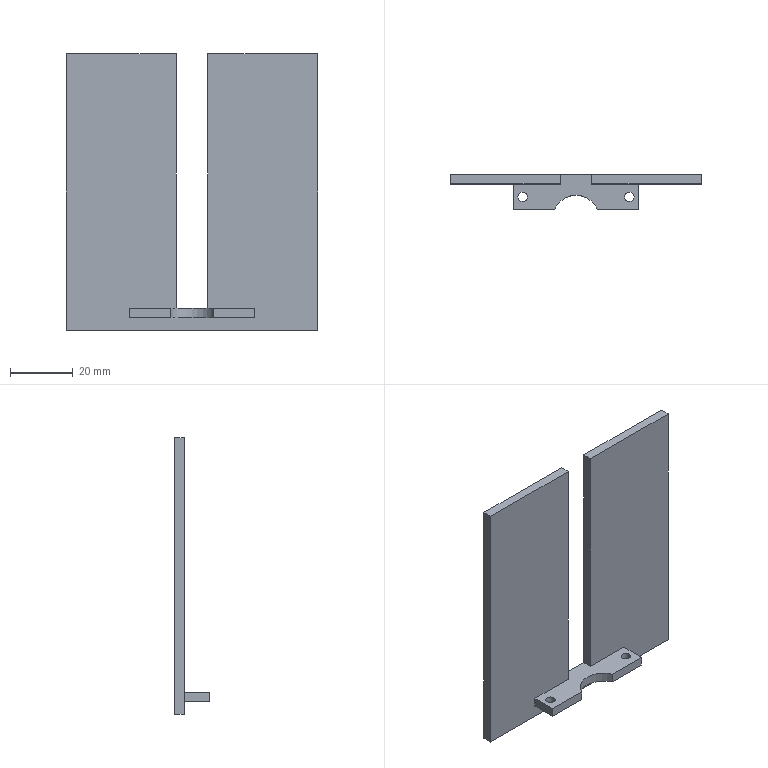Part | SolidWorks | features Extrusion 1, ICE 1 | 1 solid | 20 faces | box 80 x 11 x 88 mm | volume 19474 mm3 | plane 15 | cylinder 5 | commonest cylinder face diameters 3 x4 15 x1
STEP:
#1=CARTESIAN_POINT('',(15.5,7.,3.));
#2=VERTEX_POINT('',#1);
#3=CARTESIAN_POINT('',(18.5,7.,3.));
#4=VERTEX_POINT('',#3);
#5=CARTESIAN_POINT('',(17.,7.,3.));
#6=DIRECTION('',(0.,0.,1.));
#7=DIRECTION('',(1.,0.,0.));
#8=AXIS2_PLACEMENT_3D('',#5,#6,#7);
#9=CIRCLE('',#8,1.5);
#10=EDGE_CURVE('',#2,#4,#9,.T.);
#11=ORIENTED_EDGE('',*,*,#10,.T.);
#12=CARTESIAN_POINT('',(18.5,7.,0.));
#13=VERTEX_POINT('',#12);
#14=CARTESIAN_POINT('',(18.5,7.,3.));
#15=DIRECTION('',(0.,0.,-1.));
#16=VECTOR('',#15,1000.);
#17=LINE('',#14,#16);
#18=EDGE_CURVE('',#4,#13,#17,.T.);
#19=ORIENTED_EDGE('',*,*,#18,.T.);
#20=CARTESIAN_POINT('',(15.5,7.,0.));
#21=VERTEX_POINT('',#20);
#22=CARTESIAN_POINT('',(17.,7.,0.));
#23=DIRECTION('',(0.,0.,1.));
#24=DIRECTION('',(1.,0.,0.));
#25=AXIS2_PLACEMENT_3D('',#22,#23,#24);
#26=CIRCLE('',#25,1.5);
#27=EDGE_CURVE('',#21,#13,#26,.T.);
#28=ORIENTED_EDGE('',*,*,#27,.F.);
#29=CARTESIAN_POINT('',(15.5,7.,3.));
#30=DIRECTION('',(0.,0.,-1.));
#31=VECTOR('',#30,1000.);
#32=LINE('',#29,#31);
#33=EDGE_CURVE('',#2,#21,#32,.T.);
#34=ORIENTED_EDGE('',*,*,#33,.F.);
#35=EDGE_LOOP('',(#11,#19,#28,#34));
#36=FACE_OUTER_BOUND('',#35,.T.);
#37=CARTESIAN_POINT('',(17.,7.,3.));
#38=DIRECTION('',(0.,0.,-1.));
#39=DIRECTION('',(-1.,0.,0.));
#40=AXIS2_PLACEMENT_3D('',#37,#38,#39);
#41=CYLINDRICAL_SURFACE('',#40,1.5);
#42=ADVANCED_FACE('',(#36),#41,.F.);
#43=CARTESIAN_POINT('',(-18.5,7.,3.));
#44=VERTEX_POINT('',#43);
#45=CARTESIAN_POINT('',(-15.5,7.,3.));
#46=VERTEX_POINT('',#45);
#47=CARTESIAN_POINT('',(-17.,7.,3.));
#48=DIRECTION('',(0.,0.,1.));
#49=DIRECTION('',(1.,0.,0.));
#50=AXIS2_PLACEMENT_3D('',#47,#48,#49);
#51=CIRCLE('',#50,1.5);
#52=EDGE_CURVE('',#44,#46,#51,.T.);
#53=ORIENTED_EDGE('',*,*,#52,.T.);
#54=CARTESIAN_POINT('',(-15.5,7.,0.));
#55=VERTEX_POINT('',#54);
#56=CARTESIAN_POINT('',(-15.5,7.,3.));
#57=DIRECTION('',(0.,0.,-1.));
#58=VECTOR('',#57,1000.);
#59=LINE('',#56,#58);
#60=EDGE_CURVE('',#46,#55,#59,.T.);
#61=ORIENTED_EDGE('',*,*,#60,.T.);
#62=CARTESIAN_POINT('',(-18.5,7.,0.));
#63=VERTEX_POINT('',#62);
#64=CARTESIAN_POINT('',(-17.,7.,0.));
#65=DIRECTION('',(0.,0.,1.));
#66=DIRECTION('',(1.,0.,0.));
#67=AXIS2_PLACEMENT_3D('',#64,#65,#66);
#68=CIRCLE('',#67,1.5);
#69=EDGE_CURVE('',#63,#55,#68,.T.);
#70=ORIENTED_EDGE('',*,*,#69,.F.);
#71=CARTESIAN_POINT('',(-18.5,7.,3.));
#72=DIRECTION('',(0.,0.,-1.));
#73=VECTOR('',#72,1000.);
#74=LINE('',#71,#73);
#75=EDGE_CURVE('',#44,#63,#74,.T.);
#76=ORIENTED_EDGE('',*,*,#75,.F.);
#77=EDGE_LOOP('',(#53,#61,#70,#76));
#78=FACE_OUTER_BOUND('',#77,.T.);
#79=CARTESIAN_POINT('',(-17.,7.,3.));
#80=DIRECTION('',(0.,0.,-1.));
#81=DIRECTION('',(-1.,0.,0.));
#82=AXIS2_PLACEMENT_3D('',#79,#80,#81);
#83=CYLINDRICAL_SURFACE('',#82,1.5);
#84=ADVANCED_FACE('',(#78),#83,.F.);
#85=ORIENTED_EDGE('',*,*,#52,.F.);
#86=CARTESIAN_POINT('',(-17.,7.,3.));
#87=DIRECTION('',(0.,0.,1.));
#88=DIRECTION('',(1.,0.,0.));
#89=AXIS2_PLACEMENT_3D('',#86,#87,#88);
#90=CIRCLE('',#89,1.5);
#91=EDGE_CURVE('',#46,#44,#90,.T.);
#92=ORIENTED_EDGE('',*,*,#91,.F.);
#93=EDGE_LOOP('',(#85,#92));
#94=FACE_BOUND('',#93,.T.);
#95=CARTESIAN_POINT('',(20.,3.,3.));
#96=VERTEX_POINT('',#95);
#97=CARTESIAN_POINT('',(20.,11.,3.));
#98=VERTEX_POINT('',#97);
#99=CARTESIAN_POINT('',(20.,3.,3.));
#100=DIRECTION('',(0.,1.,0.));
#101=VECTOR('',#100,1000.);
#102=LINE('',#99,#101);
#103=EDGE_CURVE('',#96,#98,#102,.T.);
#104=ORIENTED_EDGE('',*,*,#103,.T.);
#105=CARTESIAN_POINT('',(5.,11.,3.));
#106=VERTEX_POINT('',#105);
#107=CARTESIAN_POINT('',(-20.,11.,3.));
#108=DIRECTION('',(-1.,0.,0.));
#109=VECTOR('',#108,1000.);
#110=LINE('',#107,#109);
#111=EDGE_CURVE('',#98,#106,#110,.T.);
#112=ORIENTED_EDGE('',*,*,#111,.T.);
#113=CARTESIAN_POINT('',(5.,14.,3.));
#114=VERTEX_POINT('',#113);
#115=CARTESIAN_POINT('',(5.,14.,3.));
#116=DIRECTION('',(0.,-1.,0.));
#117=VECTOR('',#116,1000.);
#118=LINE('',#115,#117);
#119=EDGE_CURVE('',#114,#106,#118,.T.);
#120=ORIENTED_EDGE('',*,*,#119,.F.);
#121=CARTESIAN_POINT('',(-5.,14.,3.));
#122=VERTEX_POINT('',#121);
#123=CARTESIAN_POINT('',(-5.,14.,3.));
#124=DIRECTION('',(1.,0.,0.));
#125=VECTOR('',#124,1000.);
#126=LINE('',#123,#125);
#127=EDGE_CURVE('',#122,#114,#126,.T.);
#128=ORIENTED_EDGE('',*,*,#127,.F.);
#129=CARTESIAN_POINT('',(-5.,11.,3.));
#130=VERTEX_POINT('',#129);
#131=CARTESIAN_POINT('',(-5.,14.,3.));
#132=DIRECTION('',(0.,-1.,0.));
#133=VECTOR('',#132,1000.);
#134=LINE('',#131,#133);
#135=EDGE_CURVE('',#122,#130,#134,.T.);
#136=ORIENTED_EDGE('',*,*,#135,.T.);
#137=CARTESIAN_POINT('',(-20.,11.,3.));
#138=VERTEX_POINT('',#137);
#139=CARTESIAN_POINT('',(-20.,11.,3.));
#140=DIRECTION('',(-1.,0.,0.));
#141=VECTOR('',#140,1000.);
#142=LINE('',#139,#141);
#143=EDGE_CURVE('',#130,#138,#142,.T.);
#144=ORIENTED_EDGE('',*,*,#143,.T.);
#145=CARTESIAN_POINT('',(-20.,3.,3.));
#146=VERTEX_POINT('',#145);
#147=CARTESIAN_POINT('',(-20.,3.,3.));
#148=DIRECTION('',(0.,-1.,0.));
#149=VECTOR('',#148,1000.);
#150=LINE('',#147,#149);
#151=EDGE_CURVE('',#138,#146,#150,.T.);
#152=ORIENTED_EDGE('',*,*,#151,.T.);
#153=CARTESIAN_POINT('',(-6.874,3.,3.));
#154=VERTEX_POINT('',#153);
#155=CARTESIAN_POINT('',(-20.,3.,3.));
#156=DIRECTION('',(1.,0.,0.));
#157=VECTOR('',#156,1000.);
#158=LINE('',#155,#157);
#159=EDGE_CURVE('',#146,#154,#158,.T.);
#160=ORIENTED_EDGE('',*,*,#159,.T.);
#161=CARTESIAN_POINT('',(6.874,3.,3.));
#162=VERTEX_POINT('',#161);
#163=CARTESIAN_POINT('',(0.,0.,3.));
#164=DIRECTION('',(0.,0.,-1.));
#165=DIRECTION('',(1.,0.,0.));
#166=AXIS2_PLACEMENT_3D('',#163,#164,#165);
#167=CIRCLE('',#166,7.5);
#168=EDGE_CURVE('',#154,#162,#167,.T.);
#169=ORIENTED_EDGE('',*,*,#168,.T.);
#170=CARTESIAN_POINT('',(6.874,3.,3.));
#171=DIRECTION('',(1.,0.,0.));
#172=VECTOR('',#171,1000.);
#173=LINE('',#170,#172);
#174=EDGE_CURVE('',#162,#96,#173,.T.);
#175=ORIENTED_EDGE('',*,*,#174,.T.);
#176=EDGE_LOOP('',(#104,#112,#120,#128,#136,#144,#152,#160,#169,#175));
#177=FACE_OUTER_BOUND('',#176,.T.);
#178=ORIENTED_EDGE('',*,*,#10,.F.);
#179=CARTESIAN_POINT('',(17.,7.,3.));
#180=DIRECTION('',(0.,0.,1.));
#181=DIRECTION('',(1.,0.,0.));
#182=AXIS2_PLACEMENT_3D('',#179,#180,#181);
#183=CIRCLE('',#182,1.5);
#184=EDGE_CURVE('',#4,#2,#183,.T.);
#185=ORIENTED_EDGE('',*,*,#184,.F.);
#186=EDGE_LOOP('',(#178,#185));
#187=FACE_BOUND('',#186,.T.);
#188=CARTESIAN_POINT('',(0.,0.,3.));
#189=DIRECTION('',(0.,0.,1.));
#190=DIRECTION('',(1.,0.,0.));
#191=AXIS2_PLACEMENT_3D('',#188,#189,#190);
#192=PLANE('',#191);
#193=ADVANCED_FACE('',(#94,#177,#187),#192,.T.);
#194=CARTESIAN_POINT('',(20.,3.,0.));
#195=VERTEX_POINT('',#194);
#196=CARTESIAN_POINT('',(20.,11.,0.));
#197=VERTEX_POINT('',#196);
#198=CARTESIAN_POINT('',(20.,3.,0.));
#199=DIRECTION('',(0.,1.,0.));
#200=VECTOR('',#199,1000.);
#201=LINE('',#198,#200);
#202=EDGE_CURVE('',#195,#197,#201,.T.);
#203=ORIENTED_EDGE('',*,*,#202,.F.);
#204=CARTESIAN_POINT('',(6.874,3.,0.));
#205=VERTEX_POINT('',#204);
#206=CARTESIAN_POINT('',(6.874,3.,0.));
#207=DIRECTION('',(1.,0.,0.));
#208=VECTOR('',#207,1000.);
#209=LINE('',#206,#208);
#210=EDGE_CURVE('',#205,#195,#209,.T.);
#211=ORIENTED_EDGE('',*,*,#210,.F.);
#212=CARTESIAN_POINT('',(-6.874,3.,0.));
#213=VERTEX_POINT('',#212);
#214=CARTESIAN_POINT('',(0.,0.,0.));
#215=DIRECTION('',(0.,0.,-1.));
#216=DIRECTION('',(1.,0.,0.));
#217=AXIS2_PLACEMENT_3D('',#214,#215,#216);
#218=CIRCLE('',#217,7.5);
#219=EDGE_CURVE('',#213,#205,#218,.T.);
#220=ORIENTED_EDGE('',*,*,#219,.F.);
#221=CARTESIAN_POINT('',(-20.,3.,0.));
#222=VERTEX_POINT('',#221);
#223=CARTESIAN_POINT('',(-20.,3.,0.));
#224=DIRECTION('',(1.,0.,0.));
#225=VECTOR('',#224,1000.);
#226=LINE('',#223,#225);
#227=EDGE_CURVE('',#222,#213,#226,.T.);
#228=ORIENTED_EDGE('',*,*,#227,.F.);
#229=CARTESIAN_POINT('',(-20.,11.,0.));
#230=VERTEX_POINT('',#229);
#231=CARTESIAN_POINT('',(-20.,3.,0.));
#232=DIRECTION('',(0.,-1.,0.));
#233=VECTOR('',#232,1000.);
#234=LINE('',#231,#233);
#235=EDGE_CURVE('',#230,#222,#234,.T.);
#236=ORIENTED_EDGE('',*,*,#235,.F.);
#237=CARTESIAN_POINT('',(-20.,11.,0.));
#238=DIRECTION('',(-1.,0.,0.));
#239=VECTOR('',#238,1000.);
#240=LINE('',#237,#239);
#241=EDGE_CURVE('',#197,#230,#240,.T.);
#242=ORIENTED_EDGE('',*,*,#241,.F.);
#243=EDGE_LOOP('',(#203,#211,#220,#228,#236,#242));
#244=FACE_OUTER_BOUND('',#243,.T.);
#245=ORIENTED_EDGE('',*,*,#69,.T.);
#246=CARTESIAN_POINT('',(-17.,7.,0.));
#247=DIRECTION('',(0.,0.,1.));
#248=DIRECTION('',(1.,0.,0.));
#249=AXIS2_PLACEMENT_3D('',#246,#247,#248);
#250=CIRCLE('',#249,1.5);
#251=EDGE_CURVE('',#55,#63,#250,.T.);
#252=ORIENTED_EDGE('',*,*,#251,.T.);
#253=EDGE_LOOP('',(#245,#252));
#254=FACE_BOUND('',#253,.T.);
#255=ORIENTED_EDGE('',*,*,#27,.T.);
#256=CARTESIAN_POINT('',(17.,7.,0.));
#257=DIRECTION('',(0.,0.,1.));
#258=DIRECTION('',(1.,0.,0.));
#259=AXIS2_PLACEMENT_3D('',#256,#257,#258);
#260=CIRCLE('',#259,1.5);
#261=EDGE_CURVE('',#13,#21,#260,.T.);
#262=ORIENTED_EDGE('',*,*,#261,.T.);
#263=EDGE_LOOP('',(#255,#262));
#264=FACE_BOUND('',#263,.T.);
#265=CARTESIAN_POINT('',(0.,0.,0.));
#266=DIRECTION('',(0.,0.,1.));
#267=DIRECTION('',(1.,0.,0.));
#268=AXIS2_PLACEMENT_3D('',#265,#266,#267);
#269=PLANE('',#268);
#270=ADVANCED_FACE('',(#244,#254,#264),#269,.F.);
#271=ORIENTED_EDGE('',*,*,#202,.T.);
#272=CARTESIAN_POINT('',(20.,11.,3.));
#273=DIRECTION('',(0.,0.,-1.));
#274=VECTOR('',#273,1000.);
#275=LINE('',#272,#274);
#276=EDGE_CURVE('',#98,#197,#275,.T.);
#277=ORIENTED_EDGE('',*,*,#276,.F.);
#278=ORIENTED_EDGE('',*,*,#103,.F.);
#279=CARTESIAN_POINT('',(20.,3.,3.));
#280=DIRECTION('',(0.,0.,-1.));
#281=VECTOR('',#280,1000.);
#282=LINE('',#279,#281);
#283=EDGE_CURVE('',#96,#195,#282,.T.);
#284=ORIENTED_EDGE('',*,*,#283,.T.);
#285=EDGE_LOOP('',(#271,#277,#278,#284));
#286=FACE_OUTER_BOUND('',#285,.T.);
#287=CARTESIAN_POINT('',(20.,3.,3.));
#288=DIRECTION('',(-1.,0.,0.));
#289=DIRECTION('',(0.,0.,1.));
#290=AXIS2_PLACEMENT_3D('',#287,#288,#289);
#291=PLANE('',#290);
#292=ADVANCED_FACE('',(#286),#291,.F.);
#293=ORIENTED_EDGE('',*,*,#235,.T.);
#294=CARTESIAN_POINT('',(-20.,3.,3.));
#295=DIRECTION('',(0.,0.,-1.));
#296=VECTOR('',#295,1000.);
#297=LINE('',#294,#296);
#298=EDGE_CURVE('',#146,#222,#297,.T.);
#299=ORIENTED_EDGE('',*,*,#298,.F.);
#300=ORIENTED_EDGE('',*,*,#151,.F.);
#301=CARTESIAN_POINT('',(-20.,11.,3.));
#302=DIRECTION('',(0.,0.,-1.));
#303=VECTOR('',#302,1000.);
#304=LINE('',#301,#303);
#305=EDGE_CURVE('',#138,#230,#304,.T.);
#306=ORIENTED_EDGE('',*,*,#305,.T.);
#307=EDGE_LOOP('',(#293,#299,#300,#306));
#308=FACE_OUTER_BOUND('',#307,.T.);
#309=CARTESIAN_POINT('',(-20.,3.,3.));
#310=DIRECTION('',(1.,0.,0.));
#311=DIRECTION('',(0.,0.,-1.));
#312=AXIS2_PLACEMENT_3D('',#309,#310,#311);
#313=PLANE('',#312);
#314=ADVANCED_FACE('',(#308),#313,.F.);
#315=ORIENTED_EDGE('',*,*,#227,.T.);
#316=CARTESIAN_POINT('',(-6.874,3.,3.));
#317=DIRECTION('',(0.,0.,-1.));
#318=VECTOR('',#317,1000.);
#319=LINE('',#316,#318);
#320=EDGE_CURVE('',#154,#213,#319,.T.);
#321=ORIENTED_EDGE('',*,*,#320,.F.);
#322=ORIENTED_EDGE('',*,*,#159,.F.);
#323=ORIENTED_EDGE('',*,*,#298,.T.);
#324=EDGE_LOOP('',(#315,#321,#322,#323));
#325=FACE_OUTER_BOUND('',#324,.T.);
#326=CARTESIAN_POINT('',(-20.,3.,3.));
#327=DIRECTION('',(0.,1.,0.));
#328=DIRECTION('',(0.,0.,1.));
#329=AXIS2_PLACEMENT_3D('',#326,#327,#328);
#330=PLANE('',#329);
#331=ADVANCED_FACE('',(#325),#330,.F.);
#332=ORIENTED_EDGE('',*,*,#219,.T.);
#333=CARTESIAN_POINT('',(6.874,3.,3.));
#334=DIRECTION('',(0.,0.,-1.));
#335=VECTOR('',#334,1000.);
#336=LINE('',#333,#335);
#337=EDGE_CURVE('',#162,#205,#336,.T.);
#338=ORIENTED_EDGE('',*,*,#337,.F.);
#339=ORIENTED_EDGE('',*,*,#168,.F.);
#340=ORIENTED_EDGE('',*,*,#320,.T.);
#341=EDGE_LOOP('',(#332,#338,#339,#340));
#342=FACE_OUTER_BOUND('',#341,.T.);
#343=CARTESIAN_POINT('',(0.,0.,3.));
#344=DIRECTION('',(0.,0.,-1.));
#345=DIRECTION('',(-1.,0.,0.));
#346=AXIS2_PLACEMENT_3D('',#343,#344,#345);
#347=CYLINDRICAL_SURFACE('',#346,7.5);
#348=ADVANCED_FACE('',(#342),#347,.F.);
#349=ORIENTED_EDGE('',*,*,#210,.T.);
#350=ORIENTED_EDGE('',*,*,#283,.F.);
#351=ORIENTED_EDGE('',*,*,#174,.F.);
#352=ORIENTED_EDGE('',*,*,#337,.T.);
#353=EDGE_LOOP('',(#349,#350,#351,#352));
#354=FACE_OUTER_BOUND('',#353,.T.);
#355=CARTESIAN_POINT('',(6.874,3.,3.));
#356=DIRECTION('',(0.,1.,0.));
#357=DIRECTION('',(0.,0.,1.));
#358=AXIS2_PLACEMENT_3D('',#355,#356,#357);
#359=PLANE('',#358);
#360=ADVANCED_FACE('',(#354),#359,.F.);
#361=ORIENTED_EDGE('',*,*,#60,.F.);
#362=ORIENTED_EDGE('',*,*,#91,.T.);
#363=ORIENTED_EDGE('',*,*,#75,.T.);
#364=ORIENTED_EDGE('',*,*,#251,.F.);
#365=EDGE_LOOP('',(#361,#362,#363,#364));
#366=FACE_OUTER_BOUND('',#365,.T.);
#367=CARTESIAN_POINT('',(-17.,7.,3.));
#368=DIRECTION('',(0.,0.,-1.));
#369=DIRECTION('',(-1.,0.,0.));
#370=AXIS2_PLACEMENT_3D('',#367,#368,#369);
#371=CYLINDRICAL_SURFACE('',#370,1.5);
#372=ADVANCED_FACE('',(#366),#371,.F.);
#373=ORIENTED_EDGE('',*,*,#18,.F.);
#374=ORIENTED_EDGE('',*,*,#184,.T.);
#375=ORIENTED_EDGE('',*,*,#33,.T.);
#376=ORIENTED_EDGE('',*,*,#261,.F.);
#377=EDGE_LOOP('',(#373,#374,#375,#376));
#378=FACE_OUTER_BOUND('',#377,.T.);
#379=CARTESIAN_POINT('',(17.,7.,3.));
#380=DIRECTION('',(0.,0.,-1.));
#381=DIRECTION('',(-1.,0.,0.));
#382=AXIS2_PLACEMENT_3D('',#379,#380,#381);
#383=CYLINDRICAL_SURFACE('',#382,1.5);
#384=ADVANCED_FACE('',(#378),#383,.F.);
#385=ORIENTED_EDGE('',*,*,#143,.F.);
#386=CARTESIAN_POINT('',(-5.,11.,84.));
#387=VERTEX_POINT('',#386);
#388=CARTESIAN_POINT('',(-5.,11.,3.));
#389=DIRECTION('',(0.,0.,-1.));
#390=VECTOR('',#389,1000.);
#391=LINE('',#388,#390);
#392=EDGE_CURVE('',#387,#130,#391,.T.);
#393=ORIENTED_EDGE('',*,*,#392,.F.);
#394=CARTESIAN_POINT('',(-40.,11.,84.));
#395=VERTEX_POINT('',#394);
#396=CARTESIAN_POINT('',(-5.,11.,84.));
#397=DIRECTION('',(1.,0.,0.));
#398=VECTOR('',#397,1000.);
#399=LINE('',#396,#398);
#400=EDGE_CURVE('',#395,#387,#399,.T.);
#401=ORIENTED_EDGE('',*,*,#400,.F.);
#402=CARTESIAN_POINT('',(-40.,11.,-4.));
#403=VERTEX_POINT('',#402);
#404=CARTESIAN_POINT('',(-40.,11.,0.));
#405=DIRECTION('',(0.,0.,1.));
#406=VECTOR('',#405,1000.);
#407=LINE('',#404,#406);
#408=EDGE_CURVE('',#403,#395,#407,.T.);
#409=ORIENTED_EDGE('',*,*,#408,.F.);
#410=CARTESIAN_POINT('',(40.,11.,-4.));
#411=VERTEX_POINT('',#410);
#412=CARTESIAN_POINT('',(-40.,11.,-4.));
#413=DIRECTION('',(-1.,0.,0.));
#414=VECTOR('',#413,1000.);
#415=LINE('',#412,#414);
#416=EDGE_CURVE('',#411,#403,#415,.T.);
#417=ORIENTED_EDGE('',*,*,#416,.F.);
#418=CARTESIAN_POINT('',(40.,11.,84.));
#419=VERTEX_POINT('',#418);
#420=CARTESIAN_POINT('',(40.,11.,0.));
#421=DIRECTION('',(0.,0.,-1.));
#422=VECTOR('',#421,1000.);
#423=LINE('',#420,#422);
#424=EDGE_CURVE('',#419,#411,#423,.T.);
#425=ORIENTED_EDGE('',*,*,#424,.F.);
#426=CARTESIAN_POINT('',(5.,11.,84.));
#427=VERTEX_POINT('',#426);
#428=CARTESIAN_POINT('',(40.,11.,84.));
#429=DIRECTION('',(1.,0.,0.));
#430=VECTOR('',#429,1000.);
#431=LINE('',#428,#430);
#432=EDGE_CURVE('',#427,#419,#431,.T.);
#433=ORIENTED_EDGE('',*,*,#432,.F.);
#434=CARTESIAN_POINT('',(5.,11.,3.));
#435=DIRECTION('',(0.,0.,1.));
#436=VECTOR('',#435,1000.);
#437=LINE('',#434,#436);
#438=EDGE_CURVE('',#106,#427,#437,.T.);
#439=ORIENTED_EDGE('',*,*,#438,.F.);
#440=ORIENTED_EDGE('',*,*,#111,.F.);
#441=ORIENTED_EDGE('',*,*,#276,.T.);
#442=ORIENTED_EDGE('',*,*,#241,.T.);
#443=ORIENTED_EDGE('',*,*,#305,.F.);
#444=EDGE_LOOP('',(#385,#393,#401,#409,#417,#425,#433,#439,#440,#441,#442,#443));
#445=FACE_OUTER_BOUND('',#444,.T.);
#446=CARTESIAN_POINT('',(0.,11.,0.));
#447=DIRECTION('',(0.,-1.,0.));
#448=DIRECTION('',(0.,0.,-1.));
#449=AXIS2_PLACEMENT_3D('',#446,#447,#448);
#450=PLANE('',#449);
#451=ADVANCED_FACE('',(#445),#450,.T.);
#452=ORIENTED_EDGE('',*,*,#416,.T.);
#453=CARTESIAN_POINT('',(-40.,14.,-4.));
#454=VERTEX_POINT('',#453);
#455=CARTESIAN_POINT('',(-40.,14.,-4.));
#456=DIRECTION('',(0.,-1.,0.));
#457=VECTOR('',#456,1000.);
#458=LINE('',#455,#457);
#459=EDGE_CURVE('',#454,#403,#458,.T.);
#460=ORIENTED_EDGE('',*,*,#459,.F.);
#461=CARTESIAN_POINT('',(40.,14.,-4.));
#462=VERTEX_POINT('',#461);
#463=CARTESIAN_POINT('',(-40.,14.,-4.));
#464=DIRECTION('',(-1.,0.,0.));
#465=VECTOR('',#464,1000.);
#466=LINE('',#463,#465);
#467=EDGE_CURVE('',#462,#454,#466,.T.);
#468=ORIENTED_EDGE('',*,*,#467,.F.);
#469=CARTESIAN_POINT('',(40.,14.,-4.));
#470=DIRECTION('',(0.,-1.,0.));
#471=VECTOR('',#470,1000.);
#472=LINE('',#469,#471);
#473=EDGE_CURVE('',#462,#411,#472,.T.);
#474=ORIENTED_EDGE('',*,*,#473,.T.);
#475=EDGE_LOOP('',(#452,#460,#468,#474));
#476=FACE_OUTER_BOUND('',#475,.T.);
#477=CARTESIAN_POINT('',(-40.,14.,-4.));
#478=DIRECTION('',(0.,0.,1.));
#479=DIRECTION('',(1.,0.,0.));
#480=AXIS2_PLACEMENT_3D('',#477,#478,#479);
#481=PLANE('',#480);
#482=ADVANCED_FACE('',(#476),#481,.F.);
#483=ORIENTED_EDGE('',*,*,#408,.T.);
#484=CARTESIAN_POINT('',(-40.,14.,84.));
#485=VERTEX_POINT('',#484);
#486=CARTESIAN_POINT('',(-40.,14.,84.));
#487=DIRECTION('',(0.,-1.,0.));
#488=VECTOR('',#487,1000.);
#489=LINE('',#486,#488);
#490=EDGE_CURVE('',#485,#395,#489,.T.);
#491=ORIENTED_EDGE('',*,*,#490,.F.);
#492=CARTESIAN_POINT('',(-40.,14.,0.));
#493=DIRECTION('',(0.,0.,1.));
#494=VECTOR('',#493,1000.);
#495=LINE('',#492,#494);
#496=EDGE_CURVE('',#454,#485,#495,.T.);
#497=ORIENTED_EDGE('',*,*,#496,.F.);
#498=ORIENTED_EDGE('',*,*,#459,.T.);
#499=EDGE_LOOP('',(#483,#491,#497,#498));
#500=FACE_OUTER_BOUND('',#499,.T.);
#501=CARTESIAN_POINT('',(-40.,14.,0.));
#502=DIRECTION('',(1.,0.,0.));
#503=DIRECTION('',(0.,0.,-1.));
#504=AXIS2_PLACEMENT_3D('',#501,#502,#503);
#505=PLANE('',#504);
#506=ADVANCED_FACE('',(#500),#505,.F.);
#507=ORIENTED_EDGE('',*,*,#400,.T.);
#508=CARTESIAN_POINT('',(-5.,14.,84.));
#509=VERTEX_POINT('',#508);
#510=CARTESIAN_POINT('',(-5.,14.,84.));
#511=DIRECTION('',(0.,-1.,0.));
#512=VECTOR('',#511,1000.);
#513=LINE('',#510,#512);
#514=EDGE_CURVE('',#509,#387,#513,.T.);
#515=ORIENTED_EDGE('',*,*,#514,.F.);
#516=CARTESIAN_POINT('',(-5.,14.,84.));
#517=DIRECTION('',(1.,0.,0.));
#518=VECTOR('',#517,1000.);
#519=LINE('',#516,#518);
#520=EDGE_CURVE('',#485,#509,#519,.T.);
#521=ORIENTED_EDGE('',*,*,#520,.F.);
#522=ORIENTED_EDGE('',*,*,#490,.T.);
#523=EDGE_LOOP('',(#507,#515,#521,#522));
#524=FACE_OUTER_BOUND('',#523,.T.);
#525=CARTESIAN_POINT('',(-5.,14.,84.));
#526=DIRECTION('',(0.,0.,-1.));
#527=DIRECTION('',(-1.,0.,0.));
#528=AXIS2_PLACEMENT_3D('',#525,#526,#527);
#529=PLANE('',#528);
#530=ADVANCED_FACE('',(#524),#529,.F.);
#531=ORIENTED_EDGE('',*,*,#392,.T.);
#532=ORIENTED_EDGE('',*,*,#135,.F.);
#533=CARTESIAN_POINT('',(-5.,14.,3.));
#534=DIRECTION('',(0.,0.,-1.));
#535=VECTOR('',#534,1000.);
#536=LINE('',#533,#535);
#537=EDGE_CURVE('',#509,#122,#536,.T.);
#538=ORIENTED_EDGE('',*,*,#537,.F.);
#539=ORIENTED_EDGE('',*,*,#514,.T.);
#540=EDGE_LOOP('',(#531,#532,#538,#539));
#541=FACE_OUTER_BOUND('',#540,.T.);
#542=CARTESIAN_POINT('',(-5.,14.,3.));
#543=DIRECTION('',(-1.,0.,0.));
#544=DIRECTION('',(0.,0.,1.));
#545=AXIS2_PLACEMENT_3D('',#542,#543,#544);
#546=PLANE('',#545);
#547=ADVANCED_FACE('',(#541),#546,.F.);
#548=ORIENTED_EDGE('',*,*,#438,.T.);
#549=CARTESIAN_POINT('',(5.,14.,84.));
#550=VERTEX_POINT('',#549);
#551=CARTESIAN_POINT('',(5.,14.,84.));
#552=DIRECTION('',(0.,-1.,0.));
#553=VECTOR('',#552,1000.);
#554=LINE('',#551,#553);
#555=EDGE_CURVE('',#550,#427,#554,.T.);
#556=ORIENTED_EDGE('',*,*,#555,.F.);
#557=CARTESIAN_POINT('',(5.,14.,3.));
#558=DIRECTION('',(0.,0.,1.));
#559=VECTOR('',#558,1000.);
#560=LINE('',#557,#559);
#561=EDGE_CURVE('',#114,#550,#560,.T.);
#562=ORIENTED_EDGE('',*,*,#561,.F.);
#563=ORIENTED_EDGE('',*,*,#119,.T.);
#564=EDGE_LOOP('',(#548,#556,#562,#563));
#565=FACE_OUTER_BOUND('',#564,.T.);
#566=CARTESIAN_POINT('',(5.,14.,3.));
#567=DIRECTION('',(1.,0.,0.));
#568=DIRECTION('',(0.,0.,-1.));
#569=AXIS2_PLACEMENT_3D('',#566,#567,#568);
#570=PLANE('',#569);
#571=ADVANCED_FACE('',(#565),#570,.F.);
#572=ORIENTED_EDGE('',*,*,#432,.T.);
#573=CARTESIAN_POINT('',(40.,14.,84.));
#574=VERTEX_POINT('',#573);
#575=CARTESIAN_POINT('',(40.,14.,84.));
#576=DIRECTION('',(0.,-1.,0.));
#577=VECTOR('',#576,1000.);
#578=LINE('',#575,#577);
#579=EDGE_CURVE('',#574,#419,#578,.T.);
#580=ORIENTED_EDGE('',*,*,#579,.F.);
#581=CARTESIAN_POINT('',(40.,14.,84.));
#582=DIRECTION('',(1.,0.,0.));
#583=VECTOR('',#582,1000.);
#584=LINE('',#581,#583);
#585=EDGE_CURVE('',#550,#574,#584,.T.);
#586=ORIENTED_EDGE('',*,*,#585,.F.);
#587=ORIENTED_EDGE('',*,*,#555,.T.);
#588=EDGE_LOOP('',(#572,#580,#586,#587));
#589=FACE_OUTER_BOUND('',#588,.T.);
#590=CARTESIAN_POINT('',(40.,14.,84.));
#591=DIRECTION('',(0.,0.,-1.));
#592=DIRECTION('',(-1.,0.,0.));
#593=AXIS2_PLACEMENT_3D('',#590,#591,#592);
#594=PLANE('',#593);
#595=ADVANCED_FACE('',(#589),#594,.F.);
#596=ORIENTED_EDGE('',*,*,#424,.T.);
#597=ORIENTED_EDGE('',*,*,#473,.F.);
#598=CARTESIAN_POINT('',(40.,14.,0.));
#599=DIRECTION('',(0.,0.,-1.));
#600=VECTOR('',#599,1000.);
#601=LINE('',#598,#600);
#602=EDGE_CURVE('',#574,#462,#601,.T.);
#603=ORIENTED_EDGE('',*,*,#602,.F.);
#604=ORIENTED_EDGE('',*,*,#579,.T.);
#605=EDGE_LOOP('',(#596,#597,#603,#604));
#606=FACE_OUTER_BOUND('',#605,.T.);
#607=CARTESIAN_POINT('',(40.,14.,0.));
#608=DIRECTION('',(-1.,0.,0.));
#609=DIRECTION('',(0.,0.,1.));
#610=AXIS2_PLACEMENT_3D('',#607,#608,#609);
#611=PLANE('',#610);
#612=ADVANCED_FACE('',(#606),#611,.F.);
#613=ORIENTED_EDGE('',*,*,#602,.T.);
#614=ORIENTED_EDGE('',*,*,#467,.T.);
#615=ORIENTED_EDGE('',*,*,#496,.T.);
#616=ORIENTED_EDGE('',*,*,#520,.T.);
#617=ORIENTED_EDGE('',*,*,#537,.T.);
#618=ORIENTED_EDGE('',*,*,#127,.T.);
#619=ORIENTED_EDGE('',*,*,#561,.T.);
#620=ORIENTED_EDGE('',*,*,#585,.T.);
#621=EDGE_LOOP('',(#613,#614,#615,#616,#617,#618,#619,#620));
#622=FACE_OUTER_BOUND('',#621,.T.);
#623=CARTESIAN_POINT('',(0.,14.,0.));
#624=DIRECTION('',(0.,-1.,0.));
#625=DIRECTION('',(0.,0.,-1.));
#626=AXIS2_PLACEMENT_3D('',#623,#624,#625);
#627=PLANE('',#626);
#628=ADVANCED_FACE('',(#622),#627,.F.);
#629=CLOSED_SHELL('',(#42,#84,#193,#270,#292,#314,#331,#348,#360,#372,#384,#451,#482,#506,#530,#547,#571,#595,#612,#628));
#630=MANIFOLD_SOLID_BREP('',#629);
#631=CARTESIAN_POINT('',(0.,0.,0.));
#632=DIRECTION('',(0.,0.,1.));
#633=DIRECTION('',(1.,0.,0.));
#634=AXIS2_PLACEMENT_3D('',#631,#632,#633);
#635=(LENGTH_UNIT()NAMED_UNIT(*)SI_UNIT(.MILLI.,.METRE.));
#636=UNCERTAINTY_MEASURE_WITH_UNIT(LENGTH_MEASURE(0.00001),#635,'','');
#637=(NAMED_UNIT(*)PLANE_ANGLE_UNIT()SI_UNIT($,.RADIAN.));
#638=(NAMED_UNIT(*)SI_UNIT($,.STERADIAN.)SOLID_ANGLE_UNIT());
#639=(GEOMETRIC_REPRESENTATION_CONTEXT(3)GLOBAL_UNCERTAINTY_ASSIGNED_CONTEXT((#636))GLOBAL_UNIT_ASSIGNED_CONTEXT((#635,#637,#638))REPRESENTATION_CONTEXT('',''));
#640=ADVANCED_BREP_SHAPE_REPRESENTATION('',(#630,#634),#639);